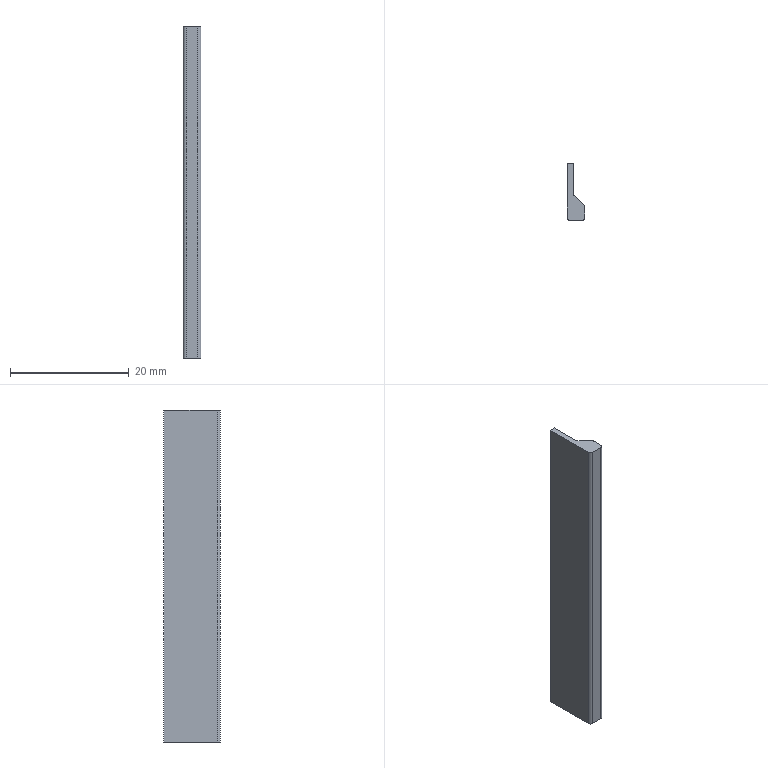Part | NX | features BREP 2 | 2 solids | 24 faces | box 3 x 9.587 x 56 mm | volume 1813 mm3 | plane 16 | cylinder 8 | commonest cylinder face diameters 1 x8
STEP:
#1=CARTESIAN_POINT('',(-0.4799,-0.2815,-4.));
#2=VERTEX_POINT('',#1);
#3=CARTESIAN_POINT('',(-0.4799,-0.2815,52.));
#4=VERTEX_POINT('',#3);
#5=CARTESIAN_POINT('',(-0.4799,-0.2815,0.));
#6=DIRECTION('',(0.,0.,1.));
#7=VECTOR('',#6,1000.);
#8=LINE('',#5,#7);
#9=EDGE_CURVE('',#2,#4,#8,.T.);
#10=ORIENTED_EDGE('',*,*,#9,.T.);
#11=CARTESIAN_POINT('',(-0.3335,-0.6351,52.));
#12=VERTEX_POINT('',#11);
#13=CARTESIAN_POINT('',(0.0201,-0.2815,52.));
#14=DIRECTION('',(0.,0.,-1.));
#15=DIRECTION('',(1.,0.,0.));
#16=AXIS2_PLACEMENT_3D('',#13,#14,#15);
#17=CIRCLE('',#16,0.5);
#18=EDGE_CURVE('',#12,#4,#17,.T.);
#19=ORIENTED_EDGE('',*,*,#18,.F.);
#20=CARTESIAN_POINT('',(-0.3335,-0.6351,-4.));
#21=VERTEX_POINT('',#20);
#22=CARTESIAN_POINT('',(-0.3335,-0.6351,0.));
#23=DIRECTION('',(0.,0.,1.));
#24=VECTOR('',#23,1000.);
#25=LINE('',#22,#24);
#26=EDGE_CURVE('',#21,#12,#25,.T.);
#27=ORIENTED_EDGE('',*,*,#26,.F.);
#28=CARTESIAN_POINT('',(0.0201,-0.2815,-4.));
#29=DIRECTION('',(0.,0.,-1.));
#30=DIRECTION('',(1.,0.,0.));
#31=AXIS2_PLACEMENT_3D('',#28,#29,#30);
#32=CIRCLE('',#31,0.5);
#33=EDGE_CURVE('',#21,#2,#32,.T.);
#34=ORIENTED_EDGE('',*,*,#33,.T.);
#35=EDGE_LOOP('',(#10,#19,#27,#34));
#36=FACE_BOUND('',#35,.T.);
#37=CARTESIAN_POINT('',(0.0201,-0.2815,0.));
#38=DIRECTION('',(0.,0.,1.));
#39=DIRECTION('',(-1.,0.,0.));
#40=AXIS2_PLACEMENT_3D('',#37,#38,#39);
#41=CYLINDRICAL_SURFACE('',#40,0.5);
#42=ADVANCED_FACE('',(#36),#41,.F.);
#43=ORIENTED_EDGE('',*,*,#26,.T.);
#44=CARTESIAN_POINT('',(1.354,-2.322,52.));
#45=VERTEX_POINT('',#44);
#46=CARTESIAN_POINT('',(-0.3335,-0.6351,52.));
#47=DIRECTION('',(-0.7071,0.7071,0.));
#48=VECTOR('',#47,1000.);
#49=LINE('',#46,#48);
#50=EDGE_CURVE('',#45,#12,#49,.T.);
#51=ORIENTED_EDGE('',*,*,#50,.F.);
#52=CARTESIAN_POINT('',(1.354,-2.322,-4.));
#53=VERTEX_POINT('',#52);
#54=CARTESIAN_POINT('',(1.354,-2.322,0.));
#55=DIRECTION('',(0.,0.,1.));
#56=VECTOR('',#55,1000.);
#57=LINE('',#54,#56);
#58=EDGE_CURVE('',#53,#45,#57,.T.);
#59=ORIENTED_EDGE('',*,*,#58,.F.);
#60=CARTESIAN_POINT('',(-0.3335,-0.6351,-4.));
#61=DIRECTION('',(-0.7071,0.7071,0.));
#62=VECTOR('',#61,1000.);
#63=LINE('',#60,#62);
#64=EDGE_CURVE('',#53,#21,#63,.T.);
#65=ORIENTED_EDGE('',*,*,#64,.T.);
#66=EDGE_LOOP('',(#43,#51,#59,#65));
#67=FACE_BOUND('',#66,.T.);
#68=CARTESIAN_POINT('',(-0.3335,-0.6351,0.));
#69=DIRECTION('',(-0.7071,-0.7071,0.));
#70=DIRECTION('',(-0.7071,0.7071,0.));
#71=AXIS2_PLACEMENT_3D('',#68,#69,#70);
#72=PLANE('',#71);
#73=ADVANCED_FACE('',(#67),#72,.F.);
#74=ORIENTED_EDGE('',*,*,#58,.T.);
#75=CARTESIAN_POINT('',(1.5,-2.676,52.));
#76=VERTEX_POINT('',#75);
#77=CARTESIAN_POINT('',(1.,-2.676,52.));
#78=DIRECTION('',(0.,0.,1.));
#79=DIRECTION('',(1.,0.,0.));
#80=AXIS2_PLACEMENT_3D('',#77,#78,#79);
#81=CIRCLE('',#80,0.5);
#82=EDGE_CURVE('',#76,#45,#81,.T.);
#83=ORIENTED_EDGE('',*,*,#82,.F.);
#84=CARTESIAN_POINT('',(1.5,-2.676,-4.));
#85=VERTEX_POINT('',#84);
#86=CARTESIAN_POINT('',(1.5,-2.676,0.));
#87=DIRECTION('',(0.,0.,1.));
#88=VECTOR('',#87,1000.);
#89=LINE('',#86,#88);
#90=EDGE_CURVE('',#85,#76,#89,.T.);
#91=ORIENTED_EDGE('',*,*,#90,.F.);
#92=CARTESIAN_POINT('',(1.,-2.676,-4.));
#93=DIRECTION('',(0.,0.,1.));
#94=DIRECTION('',(1.,0.,0.));
#95=AXIS2_PLACEMENT_3D('',#92,#93,#94);
#96=CIRCLE('',#95,0.5);
#97=EDGE_CURVE('',#85,#53,#96,.T.);
#98=ORIENTED_EDGE('',*,*,#97,.T.);
#99=EDGE_LOOP('',(#74,#83,#91,#98));
#100=FACE_BOUND('',#99,.T.);
#101=CARTESIAN_POINT('',(1.,-2.676,0.));
#102=DIRECTION('',(0.,0.,1.));
#103=DIRECTION('',(-1.,0.,0.));
#104=AXIS2_PLACEMENT_3D('',#101,#102,#103);
#105=CYLINDRICAL_SURFACE('',#104,0.5);
#106=ADVANCED_FACE('',(#100),#105,.T.);
#107=ORIENTED_EDGE('',*,*,#90,.T.);
#108=CARTESIAN_POINT('',(1.5,-4.269,52.));
#109=VERTEX_POINT('',#108);
#110=CARTESIAN_POINT('',(1.5,-6.887,52.));
#111=DIRECTION('',(0.,1.,0.));
#112=VECTOR('',#111,1000.);
#113=LINE('',#110,#112);
#114=EDGE_CURVE('',#109,#76,#113,.T.);
#115=ORIENTED_EDGE('',*,*,#114,.F.);
#116=CARTESIAN_POINT('',(1.5,-4.269,-4.));
#117=VERTEX_POINT('',#116);
#118=CARTESIAN_POINT('',(1.5,-4.269,0.));
#119=DIRECTION('',(0.,0.,1.));
#120=VECTOR('',#119,1000.);
#121=LINE('',#118,#120);
#122=EDGE_CURVE('',#117,#109,#121,.T.);
#123=ORIENTED_EDGE('',*,*,#122,.F.);
#124=CARTESIAN_POINT('',(1.5,-6.887,-4.));
#125=DIRECTION('',(0.,1.,0.));
#126=VECTOR('',#125,1000.);
#127=LINE('',#124,#126);
#128=EDGE_CURVE('',#117,#85,#127,.T.);
#129=ORIENTED_EDGE('',*,*,#128,.T.);
#130=EDGE_LOOP('',(#107,#115,#123,#129));
#131=FACE_BOUND('',#130,.T.);
#132=CARTESIAN_POINT('',(1.5,-2.676,0.));
#133=DIRECTION('',(-1.,0.,0.));
#134=DIRECTION('',(0.,1.,0.));
#135=AXIS2_PLACEMENT_3D('',#132,#133,#134);
#136=PLANE('',#135);
#137=ADVANCED_FACE('',(#131),#136,.F.);
#138=ORIENTED_EDGE('',*,*,#122,.T.);
#139=CARTESIAN_POINT('',(1.,-4.769,52.));
#140=VERTEX_POINT('',#139);
#141=CARTESIAN_POINT('',(1.,-4.269,52.));
#142=DIRECTION('',(0.,0.,1.));
#143=DIRECTION('',(1.,0.,0.));
#144=AXIS2_PLACEMENT_3D('',#141,#142,#143);
#145=CIRCLE('',#144,0.5);
#146=EDGE_CURVE('',#140,#109,#145,.T.);
#147=ORIENTED_EDGE('',*,*,#146,.F.);
#148=CARTESIAN_POINT('',(1.,-4.769,-4.));
#149=VERTEX_POINT('',#148);
#150=CARTESIAN_POINT('',(1.,-4.769,0.));
#151=DIRECTION('',(0.,0.,1.));
#152=VECTOR('',#151,1000.);
#153=LINE('',#150,#152);
#154=EDGE_CURVE('',#149,#140,#153,.T.);
#155=ORIENTED_EDGE('',*,*,#154,.F.);
#156=CARTESIAN_POINT('',(1.,-4.269,-4.));
#157=DIRECTION('',(0.,0.,1.));
#158=DIRECTION('',(1.,0.,0.));
#159=AXIS2_PLACEMENT_3D('',#156,#157,#158);
#160=CIRCLE('',#159,0.5);
#161=EDGE_CURVE('',#149,#117,#160,.T.);
#162=ORIENTED_EDGE('',*,*,#161,.T.);
#163=EDGE_LOOP('',(#138,#147,#155,#162));
#164=FACE_BOUND('',#163,.T.);
#165=CARTESIAN_POINT('',(1.,-4.269,0.));
#166=DIRECTION('',(0.,0.,1.));
#167=DIRECTION('',(-1.,0.,0.));
#168=AXIS2_PLACEMENT_3D('',#165,#166,#167);
#169=CYLINDRICAL_SURFACE('',#168,0.5);
#170=ADVANCED_FACE('',(#164),#169,.T.);
#171=ORIENTED_EDGE('',*,*,#154,.T.);
#172=CARTESIAN_POINT('',(-1.,-4.769,52.));
#173=VERTEX_POINT('',#172);
#174=CARTESIAN_POINT('',(-11.53,-4.769,52.));
#175=DIRECTION('',(1.,0.,0.));
#176=VECTOR('',#175,1000.);
#177=LINE('',#174,#176);
#178=EDGE_CURVE('',#173,#140,#177,.T.);
#179=ORIENTED_EDGE('',*,*,#178,.F.);
#180=CARTESIAN_POINT('',(-1.,-4.769,-4.));
#181=VERTEX_POINT('',#180);
#182=CARTESIAN_POINT('',(-1.,-4.769,0.));
#183=DIRECTION('',(0.,0.,1.));
#184=VECTOR('',#183,1000.);
#185=LINE('',#182,#184);
#186=EDGE_CURVE('',#181,#173,#185,.T.);
#187=ORIENTED_EDGE('',*,*,#186,.F.);
#188=CARTESIAN_POINT('',(-11.53,-4.769,-4.));
#189=DIRECTION('',(1.,0.,0.));
#190=VECTOR('',#189,1000.);
#191=LINE('',#188,#190);
#192=EDGE_CURVE('',#181,#149,#191,.T.);
#193=ORIENTED_EDGE('',*,*,#192,.T.);
#194=EDGE_LOOP('',(#171,#179,#187,#193));
#195=FACE_BOUND('',#194,.T.);
#196=CARTESIAN_POINT('',(1.,-4.769,0.));
#197=DIRECTION('',(0.,1.,0.));
#198=DIRECTION('',(1.,0.,0.));
#199=AXIS2_PLACEMENT_3D('',#196,#197,#198);
#200=PLANE('',#199);
#201=ADVANCED_FACE('',(#195),#200,.F.);
#202=ORIENTED_EDGE('',*,*,#186,.T.);
#203=CARTESIAN_POINT('',(-1.5,-4.269,52.));
#204=VERTEX_POINT('',#203);
#205=CARTESIAN_POINT('',(-1.,-4.269,52.));
#206=DIRECTION('',(0.,0.,1.));
#207=DIRECTION('',(1.,0.,0.));
#208=AXIS2_PLACEMENT_3D('',#205,#206,#207);
#209=CIRCLE('',#208,0.5);
#210=EDGE_CURVE('',#204,#173,#209,.T.);
#211=ORIENTED_EDGE('',*,*,#210,.F.);
#212=CARTESIAN_POINT('',(-1.5,-4.269,-4.));
#213=VERTEX_POINT('',#212);
#214=CARTESIAN_POINT('',(-1.5,-4.269,0.));
#215=DIRECTION('',(0.,0.,1.));
#216=VECTOR('',#215,1000.);
#217=LINE('',#214,#216);
#218=EDGE_CURVE('',#213,#204,#217,.T.);
#219=ORIENTED_EDGE('',*,*,#218,.F.);
#220=CARTESIAN_POINT('',(-1.,-4.269,-4.));
#221=DIRECTION('',(0.,0.,1.));
#222=DIRECTION('',(1.,0.,0.));
#223=AXIS2_PLACEMENT_3D('',#220,#221,#222);
#224=CIRCLE('',#223,0.5);
#225=EDGE_CURVE('',#213,#181,#224,.T.);
#226=ORIENTED_EDGE('',*,*,#225,.T.);
#227=EDGE_LOOP('',(#202,#211,#219,#226));
#228=FACE_BOUND('',#227,.T.);
#229=CARTESIAN_POINT('',(-1.,-4.269,0.));
#230=DIRECTION('',(0.,0.,1.));
#231=DIRECTION('',(-1.,0.,0.));
#232=AXIS2_PLACEMENT_3D('',#229,#230,#231);
#233=CYLINDRICAL_SURFACE('',#232,0.5);
#234=ADVANCED_FACE('',(#228),#233,.T.);
#235=ORIENTED_EDGE('',*,*,#218,.T.);
#236=CARTESIAN_POINT('',(-1.5,4.818,52.));
#237=VERTEX_POINT('',#236);
#238=CARTESIAN_POINT('',(-1.5,-6.887,52.));
#239=DIRECTION('',(0.,-1.,0.));
#240=VECTOR('',#239,1000.);
#241=LINE('',#238,#240);
#242=EDGE_CURVE('',#237,#204,#241,.T.);
#243=ORIENTED_EDGE('',*,*,#242,.F.);
#244=CARTESIAN_POINT('',(-1.5,4.818,-4.));
#245=VERTEX_POINT('',#244);
#246=CARTESIAN_POINT('',(-1.5,4.818,0.));
#247=DIRECTION('',(0.,0.,1.));
#248=VECTOR('',#247,1000.);
#249=LINE('',#246,#248);
#250=EDGE_CURVE('',#245,#237,#249,.T.);
#251=ORIENTED_EDGE('',*,*,#250,.F.);
#252=CARTESIAN_POINT('',(-1.5,-6.887,-4.));
#253=DIRECTION('',(0.,-1.,0.));
#254=VECTOR('',#253,1000.);
#255=LINE('',#252,#254);
#256=EDGE_CURVE('',#245,#213,#255,.T.);
#257=ORIENTED_EDGE('',*,*,#256,.T.);
#258=EDGE_LOOP('',(#235,#243,#251,#257));
#259=FACE_BOUND('',#258,.T.);
#260=CARTESIAN_POINT('',(-1.5,-4.269,0.));
#261=DIRECTION('',(1.,0.,0.));
#262=DIRECTION('',(0.,-1.,0.));
#263=AXIS2_PLACEMENT_3D('',#260,#261,#262);
#264=PLANE('',#263);
#265=ADVANCED_FACE('',(#259),#264,.F.);
#266=ORIENTED_EDGE('',*,*,#250,.T.);
#267=CARTESIAN_POINT('',(-0.4799,4.818,52.));
#268=VERTEX_POINT('',#267);
#269=CARTESIAN_POINT('',(-11.53,4.818,52.));
#270=DIRECTION('',(-1.,0.,0.));
#271=VECTOR('',#270,1000.);
#272=LINE('',#269,#271);
#273=EDGE_CURVE('',#268,#237,#272,.T.);
#274=ORIENTED_EDGE('',*,*,#273,.F.);
#275=CARTESIAN_POINT('',(-0.4799,4.818,-4.));
#276=VERTEX_POINT('',#275);
#277=CARTESIAN_POINT('',(-0.4799,4.818,0.));
#278=DIRECTION('',(0.,0.,1.));
#279=VECTOR('',#278,1000.);
#280=LINE('',#277,#279);
#281=EDGE_CURVE('',#276,#268,#280,.T.);
#282=ORIENTED_EDGE('',*,*,#281,.F.);
#283=CARTESIAN_POINT('',(-11.53,4.818,-4.));
#284=DIRECTION('',(-1.,0.,0.));
#285=VECTOR('',#284,1000.);
#286=LINE('',#283,#285);
#287=EDGE_CURVE('',#276,#245,#286,.T.);
#288=ORIENTED_EDGE('',*,*,#287,.T.);
#289=EDGE_LOOP('',(#266,#274,#282,#288));
#290=FACE_BOUND('',#289,.T.);
#291=CARTESIAN_POINT('',(-11.53,4.818,0.));
#292=DIRECTION('',(0.,-1.,0.));
#293=DIRECTION('',(-1.,0.,0.));
#294=AXIS2_PLACEMENT_3D('',#291,#292,#293);
#295=PLANE('',#294);
#296=ADVANCED_FACE('',(#290),#295,.F.);
#297=CARTESIAN_POINT('',(-0.4799,-6.887,-4.));
#298=DIRECTION('',(0.,1.,0.));
#299=VECTOR('',#298,1000.);
#300=LINE('',#297,#299);
#301=EDGE_CURVE('',#2,#276,#300,.T.);
#302=ORIENTED_EDGE('',*,*,#301,.T.);
#303=ORIENTED_EDGE('',*,*,#281,.T.);
#304=CARTESIAN_POINT('',(-0.4799,-6.887,52.));
#305=DIRECTION('',(0.,1.,0.));
#306=VECTOR('',#305,1000.);
#307=LINE('',#304,#306);
#308=EDGE_CURVE('',#4,#268,#307,.T.);
#309=ORIENTED_EDGE('',*,*,#308,.F.);
#310=ORIENTED_EDGE('',*,*,#9,.F.);
#311=EDGE_LOOP('',(#302,#303,#309,#310));
#312=FACE_BOUND('',#311,.T.);
#313=CARTESIAN_POINT('',(-0.4799,7.511,0.));
#314=DIRECTION('',(-1.,0.,0.));
#315=DIRECTION('',(0.,1.,0.));
#316=AXIS2_PLACEMENT_3D('',#313,#314,#315);
#317=PLANE('',#316);
#318=ADVANCED_FACE('',(#312),#317,.F.);
#319=ORIENTED_EDGE('',*,*,#273,.T.);
#320=ORIENTED_EDGE('',*,*,#242,.T.);
#321=ORIENTED_EDGE('',*,*,#210,.T.);
#322=ORIENTED_EDGE('',*,*,#178,.T.);
#323=ORIENTED_EDGE('',*,*,#146,.T.);
#324=ORIENTED_EDGE('',*,*,#114,.T.);
#325=ORIENTED_EDGE('',*,*,#82,.T.);
#326=ORIENTED_EDGE('',*,*,#50,.T.);
#327=ORIENTED_EDGE('',*,*,#18,.T.);
#328=ORIENTED_EDGE('',*,*,#308,.T.);
#329=EDGE_LOOP('',(#319,#320,#321,#322,#323,#324,#325,#326,#327,#328));
#330=FACE_BOUND('',#329,.T.);
#331=CARTESIAN_POINT('',(-11.53,-6.887,52.));
#332=DIRECTION('',(0.,0.,1.));
#333=DIRECTION('',(-1.,0.,0.));
#334=AXIS2_PLACEMENT_3D('',#331,#332,#333);
#335=PLANE('',#334);
#336=ADVANCED_FACE('',(#330),#335,.T.);
#337=ORIENTED_EDGE('',*,*,#287,.F.);
#338=ORIENTED_EDGE('',*,*,#301,.F.);
#339=ORIENTED_EDGE('',*,*,#33,.F.);
#340=ORIENTED_EDGE('',*,*,#64,.F.);
#341=ORIENTED_EDGE('',*,*,#97,.F.);
#342=ORIENTED_EDGE('',*,*,#128,.F.);
#343=ORIENTED_EDGE('',*,*,#161,.F.);
#344=ORIENTED_EDGE('',*,*,#192,.F.);
#345=ORIENTED_EDGE('',*,*,#225,.F.);
#346=ORIENTED_EDGE('',*,*,#256,.F.);
#347=EDGE_LOOP('',(#337,#338,#339,#340,#341,#342,#343,#344,#345,#346));
#348=FACE_BOUND('',#347,.T.);
#349=CARTESIAN_POINT('',(-11.53,-6.887,-4.));
#350=DIRECTION('',(0.,0.,1.));
#351=DIRECTION('',(-1.,0.,0.));
#352=AXIS2_PLACEMENT_3D('',#349,#350,#351);
#353=PLANE('',#352);
#354=ADVANCED_FACE('',(#348),#353,.F.);
#355=CLOSED_SHELL('',(#42,#73,#106,#137,#170,#201,#234,#265,#296,#318,#336,#354));
#356=MANIFOLD_SOLID_BREP('',#355);
#357=CARTESIAN_POINT('',(-0.4799,-0.2815,-4.));
#358=VERTEX_POINT('',#357);
#359=CARTESIAN_POINT('',(-0.4799,-0.2815,52.));
#360=VERTEX_POINT('',#359);
#361=CARTESIAN_POINT('',(-0.4799,-0.2815,0.));
#362=DIRECTION('',(0.,0.,1.));
#363=VECTOR('',#362,1000.);
#364=LINE('',#361,#363);
#365=EDGE_CURVE('',#358,#360,#364,.T.);
#366=ORIENTED_EDGE('',*,*,#365,.T.);
#367=CARTESIAN_POINT('',(-0.3335,-0.6351,52.));
#368=VERTEX_POINT('',#367);
#369=CARTESIAN_POINT('',(0.0201,-0.2815,52.));
#370=DIRECTION('',(0.,0.,-1.));
#371=DIRECTION('',(1.,0.,0.));
#372=AXIS2_PLACEMENT_3D('',#369,#370,#371);
#373=CIRCLE('',#372,0.5);
#374=EDGE_CURVE('',#368,#360,#373,.T.);
#375=ORIENTED_EDGE('',*,*,#374,.F.);
#376=CARTESIAN_POINT('',(-0.3335,-0.6351,-4.));
#377=VERTEX_POINT('',#376);
#378=CARTESIAN_POINT('',(-0.3335,-0.6351,0.));
#379=DIRECTION('',(0.,0.,1.));
#380=VECTOR('',#379,1000.);
#381=LINE('',#378,#380);
#382=EDGE_CURVE('',#377,#368,#381,.T.);
#383=ORIENTED_EDGE('',*,*,#382,.F.);
#384=CARTESIAN_POINT('',(0.0201,-0.2815,-4.));
#385=DIRECTION('',(0.,0.,-1.));
#386=DIRECTION('',(1.,0.,0.));
#387=AXIS2_PLACEMENT_3D('',#384,#385,#386);
#388=CIRCLE('',#387,0.5);
#389=EDGE_CURVE('',#377,#358,#388,.T.);
#390=ORIENTED_EDGE('',*,*,#389,.T.);
#391=EDGE_LOOP('',(#366,#375,#383,#390));
#392=FACE_BOUND('',#391,.T.);
#393=CARTESIAN_POINT('',(0.0201,-0.2815,0.));
#394=DIRECTION('',(0.,0.,1.));
#395=DIRECTION('',(-1.,0.,0.));
#396=AXIS2_PLACEMENT_3D('',#393,#394,#395);
#397=CYLINDRICAL_SURFACE('',#396,0.5);
#398=ADVANCED_FACE('',(#392),#397,.F.);
#399=ORIENTED_EDGE('',*,*,#382,.T.);
#400=CARTESIAN_POINT('',(1.354,-2.322,52.));
#401=VERTEX_POINT('',#400);
#402=CARTESIAN_POINT('',(-0.3335,-0.6351,52.));
#403=DIRECTION('',(-0.7071,0.7071,0.));
#404=VECTOR('',#403,1000.);
#405=LINE('',#402,#404);
#406=EDGE_CURVE('',#401,#368,#405,.T.);
#407=ORIENTED_EDGE('',*,*,#406,.F.);
#408=CARTESIAN_POINT('',(1.354,-2.322,-4.));
#409=VERTEX_POINT('',#408);
#410=CARTESIAN_POINT('',(1.354,-2.322,0.));
#411=DIRECTION('',(0.,0.,1.));
#412=VECTOR('',#411,1000.);
#413=LINE('',#410,#412);
#414=EDGE_CURVE('',#409,#401,#413,.T.);
#415=ORIENTED_EDGE('',*,*,#414,.F.);
#416=CARTESIAN_POINT('',(-0.3335,-0.6351,-4.));
#417=DIRECTION('',(-0.7071,0.7071,0.));
#418=VECTOR('',#417,1000.);
#419=LINE('',#416,#418);
#420=EDGE_CURVE('',#409,#377,#419,.T.);
#421=ORIENTED_EDGE('',*,*,#420,.T.);
#422=EDGE_LOOP('',(#399,#407,#415,#421));
#423=FACE_BOUND('',#422,.T.);
#424=CARTESIAN_POINT('',(-0.3335,-0.6351,0.));
#425=DIRECTION('',(-0.7071,-0.7071,0.));
#426=DIRECTION('',(-0.7071,0.7071,0.));
#427=AXIS2_PLACEMENT_3D('',#424,#425,#426);
#428=PLANE('',#427);
#429=ADVANCED_FACE('',(#423),#428,.F.);
#430=ORIENTED_EDGE('',*,*,#414,.T.);
#431=CARTESIAN_POINT('',(1.5,-2.676,52.));
#432=VERTEX_POINT('',#431);
#433=CARTESIAN_POINT('',(1.,-2.676,52.));
#434=DIRECTION('',(0.,0.,1.));
#435=DIRECTION('',(1.,0.,0.));
#436=AXIS2_PLACEMENT_3D('',#433,#434,#435);
#437=CIRCLE('',#436,0.5);
#438=EDGE_CURVE('',#432,#401,#437,.T.);
#439=ORIENTED_EDGE('',*,*,#438,.F.);
#440=CARTESIAN_POINT('',(1.5,-2.676,-4.));
#441=VERTEX_POINT('',#440);
#442=CARTESIAN_POINT('',(1.5,-2.676,0.));
#443=DIRECTION('',(0.,0.,1.));
#444=VECTOR('',#443,1000.);
#445=LINE('',#442,#444);
#446=EDGE_CURVE('',#441,#432,#445,.T.);
#447=ORIENTED_EDGE('',*,*,#446,.F.);
#448=CARTESIAN_POINT('',(1.,-2.676,-4.));
#449=DIRECTION('',(0.,0.,1.));
#450=DIRECTION('',(1.,0.,0.));
#451=AXIS2_PLACEMENT_3D('',#448,#449,#450);
#452=CIRCLE('',#451,0.5);
#453=EDGE_CURVE('',#441,#409,#452,.T.);
#454=ORIENTED_EDGE('',*,*,#453,.T.);
#455=EDGE_LOOP('',(#430,#439,#447,#454));
#456=FACE_BOUND('',#455,.T.);
#457=CARTESIAN_POINT('',(1.,-2.676,0.));
#458=DIRECTION('',(0.,0.,1.));
#459=DIRECTION('',(-1.,0.,0.));
#460=AXIS2_PLACEMENT_3D('',#457,#458,#459);
#461=CYLINDRICAL_SURFACE('',#460,0.5);
#462=ADVANCED_FACE('',(#456),#461,.T.);
#463=ORIENTED_EDGE('',*,*,#446,.T.);
#464=CARTESIAN_POINT('',(1.5,-4.269,52.));
#465=VERTEX_POINT('',#464);
#466=CARTESIAN_POINT('',(1.5,-6.887,52.));
#467=DIRECTION('',(0.,1.,0.));
#468=VECTOR('',#467,1000.);
#469=LINE('',#466,#468);
#470=EDGE_CURVE('',#465,#432,#469,.T.);
#471=ORIENTED_EDGE('',*,*,#470,.F.);
#472=CARTESIAN_POINT('',(1.5,-4.269,-4.));
#473=VERTEX_POINT('',#472);
#474=CARTESIAN_POINT('',(1.5,-4.269,0.));
#475=DIRECTION('',(0.,0.,1.));
#476=VECTOR('',#475,1000.);
#477=LINE('',#474,#476);
#478=EDGE_CURVE('',#473,#465,#477,.T.);
#479=ORIENTED_EDGE('',*,*,#478,.F.);
#480=CARTESIAN_POINT('',(1.5,-6.887,-4.));
#481=DIRECTION('',(0.,1.,0.));
#482=VECTOR('',#481,1000.);
#483=LINE('',#480,#482);
#484=EDGE_CURVE('',#473,#441,#483,.T.);
#485=ORIENTED_EDGE('',*,*,#484,.T.);
#486=EDGE_LOOP('',(#463,#471,#479,#485));
#487=FACE_BOUND('',#486,.T.);
#488=CARTESIAN_POINT('',(1.5,-2.676,0.));
#489=DIRECTION('',(-1.,0.,0.));
#490=DIRECTION('',(0.,1.,0.));
#491=AXIS2_PLACEMENT_3D('',#488,#489,#490);
#492=PLANE('',#491);
#493=ADVANCED_FACE('',(#487),#492,.F.);
#494=ORIENTED_EDGE('',*,*,#478,.T.);
#495=CARTESIAN_POINT('',(1.,-4.769,52.));
#496=VERTEX_POINT('',#495);
#497=CARTESIAN_POINT('',(1.,-4.269,52.));
#498=DIRECTION('',(0.,0.,1.));
#499=DIRECTION('',(1.,0.,0.));
#500=AXIS2_PLACEMENT_3D('',#497,#498,#499);
#501=CIRCLE('',#500,0.5);
#502=EDGE_CURVE('',#496,#465,#501,.T.);
#503=ORIENTED_EDGE('',*,*,#502,.F.);
#504=CARTESIAN_POINT('',(1.,-4.769,-4.));
#505=VERTEX_POINT('',#504);
#506=CARTESIAN_POINT('',(1.,-4.769,0.));
#507=DIRECTION('',(0.,0.,1.));
#508=VECTOR('',#507,1000.);
#509=LINE('',#506,#508);
#510=EDGE_CURVE('',#505,#496,#509,.T.);
#511=ORIENTED_EDGE('',*,*,#510,.F.);
#512=CARTESIAN_POINT('',(1.,-4.269,-4.));
#513=DIRECTION('',(0.,0.,1.));
#514=DIRECTION('',(1.,0.,0.));
#515=AXIS2_PLACEMENT_3D('',#512,#513,#514);
#516=CIRCLE('',#515,0.5);
#517=EDGE_CURVE('',#505,#473,#516,.T.);
#518=ORIENTED_EDGE('',*,*,#517,.T.);
#519=EDGE_LOOP('',(#494,#503,#511,#518));
#520=FACE_BOUND('',#519,.T.);
#521=CARTESIAN_POINT('',(1.,-4.269,0.));
#522=DIRECTION('',(0.,0.,1.));
#523=DIRECTION('',(-1.,0.,0.));
#524=AXIS2_PLACEMENT_3D('',#521,#522,#523);
#525=CYLINDRICAL_SURFACE('',#524,0.5);
#526=ADVANCED_FACE('',(#520),#525,.T.);
#527=ORIENTED_EDGE('',*,*,#510,.T.);
#528=CARTESIAN_POINT('',(-1.,-4.769,52.));
#529=VERTEX_POINT('',#528);
#530=CARTESIAN_POINT('',(-11.53,-4.769,52.));
#531=DIRECTION('',(1.,0.,0.));
#532=VECTOR('',#531,1000.);
#533=LINE('',#530,#532);
#534=EDGE_CURVE('',#529,#496,#533,.T.);
#535=ORIENTED_EDGE('',*,*,#534,.F.);
#536=CARTESIAN_POINT('',(-1.,-4.769,-4.));
#537=VERTEX_POINT('',#536);
#538=CARTESIAN_POINT('',(-1.,-4.769,0.));
#539=DIRECTION('',(0.,0.,1.));
#540=VECTOR('',#539,1000.);
#541=LINE('',#538,#540);
#542=EDGE_CURVE('',#537,#529,#541,.T.);
#543=ORIENTED_EDGE('',*,*,#542,.F.);
#544=CARTESIAN_POINT('',(-11.53,-4.769,-4.));
#545=DIRECTION('',(1.,0.,0.));
#546=VECTOR('',#545,1000.);
#547=LINE('',#544,#546);
#548=EDGE_CURVE('',#537,#505,#547,.T.);
#549=ORIENTED_EDGE('',*,*,#548,.T.);
#550=EDGE_LOOP('',(#527,#535,#543,#549));
#551=FACE_BOUND('',#550,.T.);
#552=CARTESIAN_POINT('',(1.,-4.769,0.));
#553=DIRECTION('',(0.,1.,0.));
#554=DIRECTION('',(1.,0.,0.));
#555=AXIS2_PLACEMENT_3D('',#552,#553,#554);
#556=PLANE('',#555);
#557=ADVANCED_FACE('',(#551),#556,.F.);
#558=ORIENTED_EDGE('',*,*,#542,.T.);
#559=CARTESIAN_POINT('',(-1.5,-4.269,52.));
#560=VERTEX_POINT('',#559);
#561=CARTESIAN_POINT('',(-1.,-4.269,52.));
#562=DIRECTION('',(0.,0.,1.));
#563=DIRECTION('',(1.,0.,0.));
#564=AXIS2_PLACEMENT_3D('',#561,#562,#563);
#565=CIRCLE('',#564,0.5);
#566=EDGE_CURVE('',#560,#529,#565,.T.);
#567=ORIENTED_EDGE('',*,*,#566,.F.);
#568=CARTESIAN_POINT('',(-1.5,-4.269,-4.));
#569=VERTEX_POINT('',#568);
#570=CARTESIAN_POINT('',(-1.5,-4.269,0.));
#571=DIRECTION('',(0.,0.,1.));
#572=VECTOR('',#571,1000.);
#573=LINE('',#570,#572);
#574=EDGE_CURVE('',#569,#560,#573,.T.);
#575=ORIENTED_EDGE('',*,*,#574,.F.);
#576=CARTESIAN_POINT('',(-1.,-4.269,-4.));
#577=DIRECTION('',(0.,0.,1.));
#578=DIRECTION('',(1.,0.,0.));
#579=AXIS2_PLACEMENT_3D('',#576,#577,#578);
#580=CIRCLE('',#579,0.5);
#581=EDGE_CURVE('',#569,#537,#580,.T.);
#582=ORIENTED_EDGE('',*,*,#581,.T.);
#583=EDGE_LOOP('',(#558,#567,#575,#582));
#584=FACE_BOUND('',#583,.T.);
#585=CARTESIAN_POINT('',(-1.,-4.269,0.));
#586=DIRECTION('',(0.,0.,1.));
#587=DIRECTION('',(-1.,0.,0.));
#588=AXIS2_PLACEMENT_3D('',#585,#586,#587);
#589=CYLINDRICAL_SURFACE('',#588,0.5);
#590=ADVANCED_FACE('',(#584),#589,.T.);
#591=ORIENTED_EDGE('',*,*,#574,.T.);
#592=CARTESIAN_POINT('',(-1.5,4.818,52.));
#593=VERTEX_POINT('',#592);
#594=CARTESIAN_POINT('',(-1.5,-6.887,52.));
#595=DIRECTION('',(0.,-1.,0.));
#596=VECTOR('',#595,1000.);
#597=LINE('',#594,#596);
#598=EDGE_CURVE('',#593,#560,#597,.T.);
#599=ORIENTED_EDGE('',*,*,#598,.F.);
#600=CARTESIAN_POINT('',(-1.5,4.818,-4.));
#601=VERTEX_POINT('',#600);
#602=CARTESIAN_POINT('',(-1.5,4.818,0.));
#603=DIRECTION('',(0.,0.,1.));
#604=VECTOR('',#603,1000.);
#605=LINE('',#602,#604);
#606=EDGE_CURVE('',#601,#593,#605,.T.);
#607=ORIENTED_EDGE('',*,*,#606,.F.);
#608=CARTESIAN_POINT('',(-1.5,-6.887,-4.));
#609=DIRECTION('',(0.,-1.,0.));
#610=VECTOR('',#609,1000.);
#611=LINE('',#608,#610);
#612=EDGE_CURVE('',#601,#569,#611,.T.);
#613=ORIENTED_EDGE('',*,*,#612,.T.);
#614=EDGE_LOOP('',(#591,#599,#607,#613));
#615=FACE_BOUND('',#614,.T.);
#616=CARTESIAN_POINT('',(-1.5,-4.269,0.));
#617=DIRECTION('',(1.,0.,0.));
#618=DIRECTION('',(0.,-1.,0.));
#619=AXIS2_PLACEMENT_3D('',#616,#617,#618);
#620=PLANE('',#619);
#621=ADVANCED_FACE('',(#615),#620,.F.);
#622=ORIENTED_EDGE('',*,*,#606,.T.);
#623=CARTESIAN_POINT('',(-0.4799,4.818,52.));
#624=VERTEX_POINT('',#623);
#625=CARTESIAN_POINT('',(-11.53,4.818,52.));
#626=DIRECTION('',(-1.,0.,0.));
#627=VECTOR('',#626,1000.);
#628=LINE('',#625,#627);
#629=EDGE_CURVE('',#624,#593,#628,.T.);
#630=ORIENTED_EDGE('',*,*,#629,.F.);
#631=CARTESIAN_POINT('',(-0.4799,4.818,-4.));
#632=VERTEX_POINT('',#631);
#633=CARTESIAN_POINT('',(-0.4799,4.818,0.));
#634=DIRECTION('',(0.,0.,1.));
#635=VECTOR('',#634,1000.);
#636=LINE('',#633,#635);
#637=EDGE_CURVE('',#632,#624,#636,.T.);
#638=ORIENTED_EDGE('',*,*,#637,.F.);
#639=CARTESIAN_POINT('',(-11.53,4.818,-4.));
#640=DIRECTION('',(-1.,0.,0.));
#641=VECTOR('',#640,1000.);
#642=LINE('',#639,#641);
#643=EDGE_CURVE('',#632,#601,#642,.T.);
#644=ORIENTED_EDGE('',*,*,#643,.T.);
#645=EDGE_LOOP('',(#622,#630,#638,#644));
#646=FACE_BOUND('',#645,.T.);
#647=CARTESIAN_POINT('',(-11.53,4.818,0.));
#648=DIRECTION('',(0.,-1.,0.));
#649=DIRECTION('',(-1.,0.,0.));
#650=AXIS2_PLACEMENT_3D('',#647,#648,#649);
#651=PLANE('',#650);
#652=ADVANCED_FACE('',(#646),#651,.F.);
#653=CARTESIAN_POINT('',(-0.4799,-6.887,-4.));
#654=DIRECTION('',(0.,1.,0.));
#655=VECTOR('',#654,1000.);
#656=LINE('',#653,#655);
#657=EDGE_CURVE('',#358,#632,#656,.T.);
#658=ORIENTED_EDGE('',*,*,#657,.T.);
#659=ORIENTED_EDGE('',*,*,#637,.T.);
#660=CARTESIAN_POINT('',(-0.4799,-6.887,52.));
#661=DIRECTION('',(0.,1.,0.));
#662=VECTOR('',#661,1000.);
#663=LINE('',#660,#662);
#664=EDGE_CURVE('',#360,#624,#663,.T.);
#665=ORIENTED_EDGE('',*,*,#664,.F.);
#666=ORIENTED_EDGE('',*,*,#365,.F.);
#667=EDGE_LOOP('',(#658,#659,#665,#666));
#668=FACE_BOUND('',#667,.T.);
#669=CARTESIAN_POINT('',(-0.4799,7.511,0.));
#670=DIRECTION('',(-1.,0.,0.));
#671=DIRECTION('',(0.,1.,0.));
#672=AXIS2_PLACEMENT_3D('',#669,#670,#671);
#673=PLANE('',#672);
#674=ADVANCED_FACE('',(#668),#673,.F.);
#675=ORIENTED_EDGE('',*,*,#629,.T.);
#676=ORIENTED_EDGE('',*,*,#598,.T.);
#677=ORIENTED_EDGE('',*,*,#566,.T.);
#678=ORIENTED_EDGE('',*,*,#534,.T.);
#679=ORIENTED_EDGE('',*,*,#502,.T.);
#680=ORIENTED_EDGE('',*,*,#470,.T.);
#681=ORIENTED_EDGE('',*,*,#438,.T.);
#682=ORIENTED_EDGE('',*,*,#406,.T.);
#683=ORIENTED_EDGE('',*,*,#374,.T.);
#684=ORIENTED_EDGE('',*,*,#664,.T.);
#685=EDGE_LOOP('',(#675,#676,#677,#678,#679,#680,#681,#682,#683,#684));
#686=FACE_BOUND('',#685,.T.);
#687=CARTESIAN_POINT('',(-11.53,-6.887,52.));
#688=DIRECTION('',(0.,0.,1.));
#689=DIRECTION('',(-1.,0.,0.));
#690=AXIS2_PLACEMENT_3D('',#687,#688,#689);
#691=PLANE('',#690);
#692=ADVANCED_FACE('',(#686),#691,.T.);
#693=ORIENTED_EDGE('',*,*,#643,.F.);
#694=ORIENTED_EDGE('',*,*,#657,.F.);
#695=ORIENTED_EDGE('',*,*,#389,.F.);
#696=ORIENTED_EDGE('',*,*,#420,.F.);
#697=ORIENTED_EDGE('',*,*,#453,.F.);
#698=ORIENTED_EDGE('',*,*,#484,.F.);
#699=ORIENTED_EDGE('',*,*,#517,.F.);
#700=ORIENTED_EDGE('',*,*,#548,.F.);
#701=ORIENTED_EDGE('',*,*,#581,.F.);
#702=ORIENTED_EDGE('',*,*,#612,.F.);
#703=EDGE_LOOP('',(#693,#694,#695,#696,#697,#698,#699,#700,#701,#702));
#704=FACE_BOUND('',#703,.T.);
#705=CARTESIAN_POINT('',(-11.53,-6.887,-4.));
#706=DIRECTION('',(0.,0.,1.));
#707=DIRECTION('',(-1.,0.,0.));
#708=AXIS2_PLACEMENT_3D('',#705,#706,#707);
#709=PLANE('',#708);
#710=ADVANCED_FACE('',(#704),#709,.F.);
#711=CLOSED_SHELL('',(#398,#429,#462,#493,#526,#557,#590,#621,#652,#674,#692,#710));
#712=MANIFOLD_SOLID_BREP('',#711);
#713=(LENGTH_UNIT()NAMED_UNIT(*)SI_UNIT(.MILLI.,.METRE.));
#714=UNCERTAINTY_MEASURE_WITH_UNIT(LENGTH_MEASURE(0.00001),#713,'','');
#715=(NAMED_UNIT(*)PLANE_ANGLE_UNIT()SI_UNIT($,.RADIAN.));
#716=(NAMED_UNIT(*)SI_UNIT($,.STERADIAN.)SOLID_ANGLE_UNIT());
#717=(GEOMETRIC_REPRESENTATION_CONTEXT(3)GLOBAL_UNCERTAINTY_ASSIGNED_CONTEXT((#714))GLOBAL_UNIT_ASSIGNED_CONTEXT((#713,#715,#716))REPRESENTATION_CONTEXT('',''));
#718=ADVANCED_BREP_SHAPE_REPRESENTATION('',(#356,#712),#717);